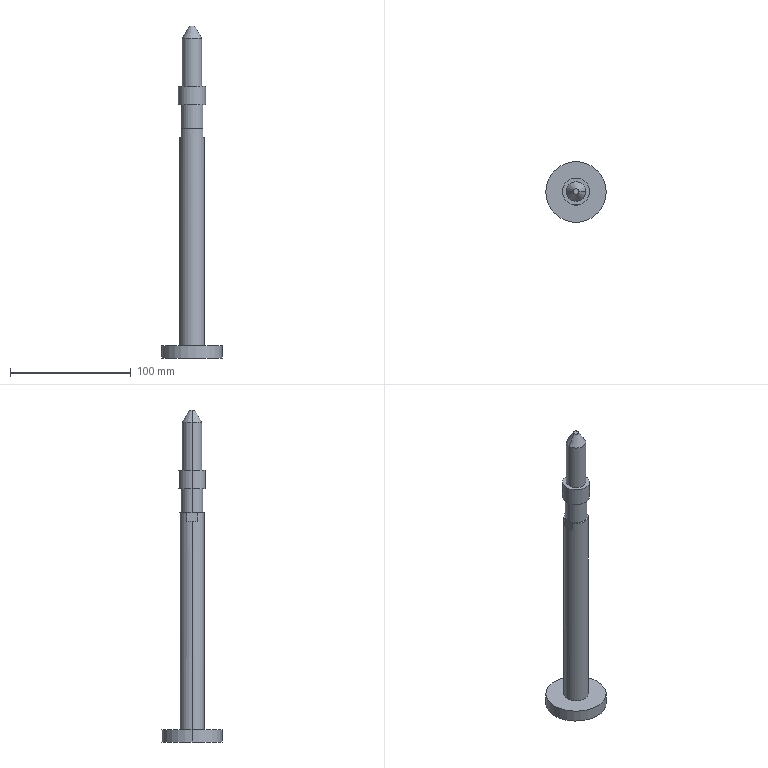Part | STEP file | MB50_125_ROD | 1 solid | 23 faces | box 50 x 50 x 274.5 mm | volume 96086 mm3 | plane 11 | cylinder 10 | cone 2 | commonest cylinder face diameters 16.16 x2 18 x2 20 x2 22.404 x2 50 x2
STEP:
#1=CARTESIAN_POINT('',(0.,0.,0.));
#2=DIRECTION('',(0.,0.,1.));
#3=DIRECTION('',(1.,0.,0.));
#4=AXIS2_PLACEMENT_3D('',#1,#2,#3);
#5=CARTESIAN_POINT('',(2.306,0.,108.));
#6=VERTEX_POINT('',#5);
#7=CARTESIAN_POINT('',(-2.306,0.,108.));
#8=VERTEX_POINT('',#7);
#9=CARTESIAN_POINT('',(0.,0.,108.));
#10=DIRECTION('',(0.,0.,1.));
#11=DIRECTION('',(1.,0.,0.));
#12=AXIS2_PLACEMENT_3D('',#9,#10,#11);
#13=CIRCLE('',#12,2.306);
#14=CARTESIAN_POINT('',(0.,0.,108.));
#15=DIRECTION('',(0.,0.,-1.));
#16=DIRECTION('',(-1.,0.,0.));
#17=AXIS2_PLACEMENT_3D('',#14,#15,#16);
#18=CONICAL_SURFACE('',#17,2.306,0.5236);
#19=CARTESIAN_POINT('',(3.142,0.));
#20=DIRECTION('',(-1.,0.));
#21=VECTOR('',#20,1.);
#22=LINE('',#19,#21);
#23=(GEOMETRIC_REPRESENTATION_CONTEXT(2)PARAMETRIC_REPRESENTATION_CONTEXT()REPRESENTATION_CONTEXT('',''));
#24=DEFINITIONAL_REPRESENTATION('',(#22),#23);
#25=PCURVE('',#18,#24);
#26=CARTESIAN_POINT('',(0.,0.,108.));
#27=DIRECTION('',(0.,0.,1.));
#28=DIRECTION('',(1.,0.,0.));
#29=AXIS2_PLACEMENT_3D('',#26,#27,#28);
#30=PLANE('',#29);
#31=CARTESIAN_POINT('',(0.,0.));
#32=DIRECTION('',(1.,0.));
#33=AXIS2_PLACEMENT_2D('',#31,#32);
#34=CIRCLE('',#33,2.306);
#35=(GEOMETRIC_REPRESENTATION_CONTEXT(2)PARAMETRIC_REPRESENTATION_CONTEXT()REPRESENTATION_CONTEXT('',''));
#36=DEFINITIONAL_REPRESENTATION('',(#34),#35);
#37=PCURVE('',#30,#36);
#38=SURFACE_CURVE('',#13,(#25,#37),.PCURVE_S1.);
#39=EDGE_CURVE('',#6,#8,#38,.T.);
#40=ORIENTED_EDGE('',*,*,#39,.F.);
#41=CARTESIAN_POINT('',(8.08,0.,98.));
#42=VERTEX_POINT('',#41);
#43=CARTESIAN_POINT('',(2.306,0.,108.));
#44=DIRECTION('',(0.5,0.,-0.866));
#45=VECTOR('',#44,1.);
#46=LINE('',#43,#45);
#47=CARTESIAN_POINT('',(3.142,0.));
#48=DIRECTION('',(0.,1.));
#49=VECTOR('',#48,1.);
#50=LINE('',#47,#49);
#51=(GEOMETRIC_REPRESENTATION_CONTEXT(2)PARAMETRIC_REPRESENTATION_CONTEXT()REPRESENTATION_CONTEXT('',''));
#52=DEFINITIONAL_REPRESENTATION('',(#50),#51);
#53=PCURVE('',#18,#52);
#54=CARTESIAN_POINT('',(0.,0.,108.));
#55=DIRECTION('',(0.,0.,-1.));
#56=DIRECTION('',(-1.,0.,0.));
#57=AXIS2_PLACEMENT_3D('',#54,#55,#56);
#58=CONICAL_SURFACE('',#57,2.306,0.5236);
#59=CARTESIAN_POINT('',(3.142,0.));
#60=DIRECTION('',(0.,1.));
#61=VECTOR('',#60,1.);
#62=LINE('',#59,#61);
#63=(GEOMETRIC_REPRESENTATION_CONTEXT(2)PARAMETRIC_REPRESENTATION_CONTEXT()REPRESENTATION_CONTEXT('',''));
#64=DEFINITIONAL_REPRESENTATION('',(#62),#63);
#65=PCURVE('',#58,#64);
#66=SURFACE_CURVE('',#46,(#53,#65),.PCURVE_S1.);
#67=EDGE_CURVE('',#6,#42,#66,.T.);
#68=ORIENTED_EDGE('',*,*,#67,.T.);
#69=CARTESIAN_POINT('',(-8.08,0.,98.));
#70=VERTEX_POINT('',#69);
#71=CARTESIAN_POINT('',(0.,0.,98.));
#72=DIRECTION('',(0.,0.,-1.));
#73=DIRECTION('',(1.,0.,0.));
#74=AXIS2_PLACEMENT_3D('',#71,#72,#73);
#75=CIRCLE('',#74,8.08);
#76=CARTESIAN_POINT('',(-3.142,10.));
#77=DIRECTION('',(1.,0.));
#78=VECTOR('',#77,1.);
#79=LINE('',#76,#78);
#80=(GEOMETRIC_REPRESENTATION_CONTEXT(2)PARAMETRIC_REPRESENTATION_CONTEXT()REPRESENTATION_CONTEXT('',''));
#81=DEFINITIONAL_REPRESENTATION('',(#79),#80);
#82=PCURVE('',#18,#81);
#83=CARTESIAN_POINT('',(0.,0.,108.));
#84=DIRECTION('',(0.,0.,-1.));
#85=DIRECTION('',(-1.,0.,0.));
#86=AXIS2_PLACEMENT_3D('',#83,#84,#85);
#87=CYLINDRICAL_SURFACE('',#86,8.08);
#88=CARTESIAN_POINT('',(-3.142,10.));
#89=DIRECTION('',(1.,0.));
#90=VECTOR('',#89,1.);
#91=LINE('',#88,#90);
#92=(GEOMETRIC_REPRESENTATION_CONTEXT(2)PARAMETRIC_REPRESENTATION_CONTEXT()REPRESENTATION_CONTEXT('',''));
#93=DEFINITIONAL_REPRESENTATION('',(#91),#92);
#94=PCURVE('',#87,#93);
#95=SURFACE_CURVE('',#75,(#82,#94),.PCURVE_S1.);
#96=EDGE_CURVE('',#70,#42,#95,.T.);
#97=ORIENTED_EDGE('',*,*,#96,.F.);
#98=CARTESIAN_POINT('',(-2.306,0.,108.));
#99=DIRECTION('',(-0.5,0.,-0.866));
#100=VECTOR('',#99,1.);
#101=LINE('',#98,#100);
#102=CARTESIAN_POINT('',(0.,0.));
#103=DIRECTION('',(0.,1.));
#104=VECTOR('',#103,1.);
#105=LINE('',#102,#104);
#106=(GEOMETRIC_REPRESENTATION_CONTEXT(2)PARAMETRIC_REPRESENTATION_CONTEXT()REPRESENTATION_CONTEXT('',''));
#107=DEFINITIONAL_REPRESENTATION('',(#105),#106);
#108=PCURVE('',#18,#107);
#109=CARTESIAN_POINT('',(6.283,0.));
#110=DIRECTION('',(0.,1.));
#111=VECTOR('',#110,1.);
#112=LINE('',#109,#111);
#113=(GEOMETRIC_REPRESENTATION_CONTEXT(2)PARAMETRIC_REPRESENTATION_CONTEXT()REPRESENTATION_CONTEXT('',''));
#114=DEFINITIONAL_REPRESENTATION('',(#112),#113);
#115=PCURVE('',#58,#114);
#116=SURFACE_CURVE('',#101,(#108,#115),.PCURVE_S1.);
#117=EDGE_CURVE('',#8,#70,#116,.T.);
#118=ORIENTED_EDGE('',*,*,#117,.F.);
#119=EDGE_LOOP('',(#40,#68,#97,#118));
#120=FACE_BOUND('',#119,.T.);
#121=ADVANCED_FACE('',(#120),#18,.T.);
#122=ORIENTED_EDGE('',*,*,#96,.T.);
#123=CARTESIAN_POINT('',(8.08,0.,58.));
#124=VERTEX_POINT('',#123);
#125=CARTESIAN_POINT('',(8.08,0.,108.));
#126=DIRECTION('',(0.,0.,-1.));
#127=VECTOR('',#126,1.);
#128=LINE('',#125,#127);
#129=CARTESIAN_POINT('',(3.142,0.));
#130=DIRECTION('',(0.,1.));
#131=VECTOR('',#130,1.);
#132=LINE('',#129,#131);
#133=(GEOMETRIC_REPRESENTATION_CONTEXT(2)PARAMETRIC_REPRESENTATION_CONTEXT()REPRESENTATION_CONTEXT('',''));
#134=DEFINITIONAL_REPRESENTATION('',(#132),#133);
#135=PCURVE('',#87,#134);
#136=CARTESIAN_POINT('',(0.,0.,108.));
#137=DIRECTION('',(0.,0.,-1.));
#138=DIRECTION('',(-1.,0.,0.));
#139=AXIS2_PLACEMENT_3D('',#136,#137,#138);
#140=CYLINDRICAL_SURFACE('',#139,8.08);
#141=CARTESIAN_POINT('',(3.142,0.));
#142=DIRECTION('',(0.,1.));
#143=VECTOR('',#142,1.);
#144=LINE('',#141,#143);
#145=(GEOMETRIC_REPRESENTATION_CONTEXT(2)PARAMETRIC_REPRESENTATION_CONTEXT()REPRESENTATION_CONTEXT('',''));
#146=DEFINITIONAL_REPRESENTATION('',(#144),#145);
#147=PCURVE('',#140,#146);
#148=SURFACE_CURVE('',#128,(#135,#147),.PCURVE_S1.);
#149=EDGE_CURVE('',#42,#124,#148,.T.);
#150=ORIENTED_EDGE('',*,*,#149,.T.);
#151=CARTESIAN_POINT('',(-8.08,0.,58.));
#152=VERTEX_POINT('',#151);
#153=CARTESIAN_POINT('',(0.,0.,58.));
#154=DIRECTION('',(0.,0.,1.));
#155=DIRECTION('',(1.,0.,0.));
#156=AXIS2_PLACEMENT_3D('',#153,#154,#155);
#157=CIRCLE('',#156,8.08);
#158=CARTESIAN_POINT('',(3.142,50.));
#159=DIRECTION('',(-1.,0.));
#160=VECTOR('',#159,1.);
#161=LINE('',#158,#160);
#162=(GEOMETRIC_REPRESENTATION_CONTEXT(2)PARAMETRIC_REPRESENTATION_CONTEXT()REPRESENTATION_CONTEXT('',''));
#163=DEFINITIONAL_REPRESENTATION('',(#161),#162);
#164=PCURVE('',#87,#163);
#165=CARTESIAN_POINT('',(0.,0.,58.));
#166=DIRECTION('',(0.,0.,1.));
#167=DIRECTION('',(1.,0.,0.));
#168=AXIS2_PLACEMENT_3D('',#165,#166,#167);
#169=PLANE('',#168);
#170=CARTESIAN_POINT('',(0.,0.));
#171=DIRECTION('',(1.,0.));
#172=AXIS2_PLACEMENT_2D('',#170,#171);
#173=CIRCLE('',#172,8.08);
#174=(GEOMETRIC_REPRESENTATION_CONTEXT(2)PARAMETRIC_REPRESENTATION_CONTEXT()REPRESENTATION_CONTEXT('',''));
#175=DEFINITIONAL_REPRESENTATION('',(#173),#174);
#176=PCURVE('',#169,#175);
#177=SURFACE_CURVE('',#157,(#164,#176),.PCURVE_S1.);
#178=EDGE_CURVE('',#124,#152,#177,.T.);
#179=ORIENTED_EDGE('',*,*,#178,.T.);
#180=CARTESIAN_POINT('',(-8.08,0.,108.));
#181=DIRECTION('',(0.,0.,-1.));
#182=VECTOR('',#181,1.);
#183=LINE('',#180,#182);
#184=CARTESIAN_POINT('',(0.,0.));
#185=DIRECTION('',(0.,1.));
#186=VECTOR('',#185,1.);
#187=LINE('',#184,#186);
#188=(GEOMETRIC_REPRESENTATION_CONTEXT(2)PARAMETRIC_REPRESENTATION_CONTEXT()REPRESENTATION_CONTEXT('',''));
#189=DEFINITIONAL_REPRESENTATION('',(#187),#188);
#190=PCURVE('',#87,#189);
#191=CARTESIAN_POINT('',(6.283,0.));
#192=DIRECTION('',(0.,1.));
#193=VECTOR('',#192,1.);
#194=LINE('',#191,#193);
#195=(GEOMETRIC_REPRESENTATION_CONTEXT(2)PARAMETRIC_REPRESENTATION_CONTEXT()REPRESENTATION_CONTEXT('',''));
#196=DEFINITIONAL_REPRESENTATION('',(#194),#195);
#197=PCURVE('',#140,#196);
#198=SURFACE_CURVE('',#183,(#190,#197),.PCURVE_S1.);
#199=EDGE_CURVE('',#70,#152,#198,.T.);
#200=ORIENTED_EDGE('',*,*,#199,.F.);
#201=EDGE_LOOP('',(#122,#150,#179,#200));
#202=FACE_BOUND('',#201,.T.);
#203=ADVANCED_FACE('',(#202),#87,.T.);
#204=CARTESIAN_POINT('',(11.202,0.,43.));
#205=VERTEX_POINT('',#204);
#206=CARTESIAN_POINT('',(-11.202,0.,43.));
#207=VERTEX_POINT('',#206);
#208=CARTESIAN_POINT('',(0.,0.,43.));
#209=DIRECTION('',(0.,0.,1.));
#210=DIRECTION('',(1.,0.,0.));
#211=AXIS2_PLACEMENT_3D('',#208,#209,#210);
#212=CIRCLE('',#211,11.202);
#213=CARTESIAN_POINT('',(0.,0.,43.));
#214=DIRECTION('',(0.,0.,1.));
#215=DIRECTION('',(1.,0.,0.));
#216=AXIS2_PLACEMENT_3D('',#213,#214,#215);
#217=CYLINDRICAL_SURFACE('',#216,11.202);
#218=CARTESIAN_POINT('',(0.,0.));
#219=DIRECTION('',(1.,0.));
#220=VECTOR('',#219,1.);
#221=LINE('',#218,#220);
#222=(GEOMETRIC_REPRESENTATION_CONTEXT(2)PARAMETRIC_REPRESENTATION_CONTEXT()REPRESENTATION_CONTEXT('',''));
#223=DEFINITIONAL_REPRESENTATION('',(#221),#222);
#224=PCURVE('',#217,#223);
#225=CARTESIAN_POINT('',(0.,0.,43.));
#226=DIRECTION('',(0.,0.,1.));
#227=DIRECTION('',(1.,0.,0.));
#228=AXIS2_PLACEMENT_3D('',#225,#226,#227);
#229=PLANE('',#228);
#230=CARTESIAN_POINT('',(0.,0.));
#231=DIRECTION('',(1.,0.));
#232=AXIS2_PLACEMENT_2D('',#230,#231);
#233=CIRCLE('',#232,11.202);
#234=(GEOMETRIC_REPRESENTATION_CONTEXT(2)PARAMETRIC_REPRESENTATION_CONTEXT()REPRESENTATION_CONTEXT('',''));
#235=DEFINITIONAL_REPRESENTATION('',(#233),#234);
#236=PCURVE('',#229,#235);
#237=SURFACE_CURVE('',#212,(#224,#236),.PCURVE_S1.);
#238=EDGE_CURVE('',#205,#207,#237,.T.);
#239=ORIENTED_EDGE('',*,*,#238,.T.);
#240=CARTESIAN_POINT('',(-11.202,0.,58.));
#241=VERTEX_POINT('',#240);
#242=CARTESIAN_POINT('',(-11.202,0.,43.));
#243=DIRECTION('',(0.,0.,1.));
#244=VECTOR('',#243,1.);
#245=LINE('',#242,#244);
#246=CARTESIAN_POINT('',(3.142,0.));
#247=DIRECTION('',(0.,1.));
#248=VECTOR('',#247,1.);
#249=LINE('',#246,#248);
#250=(GEOMETRIC_REPRESENTATION_CONTEXT(2)PARAMETRIC_REPRESENTATION_CONTEXT()REPRESENTATION_CONTEXT('',''));
#251=DEFINITIONAL_REPRESENTATION('',(#249),#250);
#252=PCURVE('',#217,#251);
#253=CARTESIAN_POINT('',(0.,0.,43.));
#254=DIRECTION('',(0.,0.,1.));
#255=DIRECTION('',(1.,0.,0.));
#256=AXIS2_PLACEMENT_3D('',#253,#254,#255);
#257=CYLINDRICAL_SURFACE('',#256,11.202);
#258=CARTESIAN_POINT('',(3.142,0.));
#259=DIRECTION('',(0.,1.));
#260=VECTOR('',#259,1.);
#261=LINE('',#258,#260);
#262=(GEOMETRIC_REPRESENTATION_CONTEXT(2)PARAMETRIC_REPRESENTATION_CONTEXT()REPRESENTATION_CONTEXT('',''));
#263=DEFINITIONAL_REPRESENTATION('',(#261),#262);
#264=PCURVE('',#257,#263);
#265=SURFACE_CURVE('',#245,(#252,#264),.PCURVE_S1.);
#266=EDGE_CURVE('',#207,#241,#265,.T.);
#267=ORIENTED_EDGE('',*,*,#266,.T.);
#268=CARTESIAN_POINT('',(11.202,0.,58.));
#269=VERTEX_POINT('',#268);
#270=CARTESIAN_POINT('',(0.,0.,58.));
#271=DIRECTION('',(0.,0.,1.));
#272=DIRECTION('',(1.,0.,0.));
#273=AXIS2_PLACEMENT_3D('',#270,#271,#272);
#274=CIRCLE('',#273,11.202);
#275=CARTESIAN_POINT('',(0.,15.));
#276=DIRECTION('',(1.,0.));
#277=VECTOR('',#276,1.);
#278=LINE('',#275,#277);
#279=(GEOMETRIC_REPRESENTATION_CONTEXT(2)PARAMETRIC_REPRESENTATION_CONTEXT()REPRESENTATION_CONTEXT('',''));
#280=DEFINITIONAL_REPRESENTATION('',(#278),#279);
#281=PCURVE('',#217,#280);
#282=CARTESIAN_POINT('',(0.,0.));
#283=DIRECTION('',(1.,0.));
#284=AXIS2_PLACEMENT_2D('',#282,#283);
#285=CIRCLE('',#284,11.202);
#286=(GEOMETRIC_REPRESENTATION_CONTEXT(2)PARAMETRIC_REPRESENTATION_CONTEXT()REPRESENTATION_CONTEXT('',''));
#287=DEFINITIONAL_REPRESENTATION('',(#285),#286);
#288=PCURVE('',#169,#287);
#289=SURFACE_CURVE('',#274,(#281,#288),.PCURVE_S1.);
#290=EDGE_CURVE('',#269,#241,#289,.T.);
#291=ORIENTED_EDGE('',*,*,#290,.F.);
#292=CARTESIAN_POINT('',(11.202,0.,43.));
#293=DIRECTION('',(0.,0.,1.));
#294=VECTOR('',#293,1.);
#295=LINE('',#292,#294);
#296=CARTESIAN_POINT('',(0.,0.));
#297=DIRECTION('',(0.,1.));
#298=VECTOR('',#297,1.);
#299=LINE('',#296,#298);
#300=(GEOMETRIC_REPRESENTATION_CONTEXT(2)PARAMETRIC_REPRESENTATION_CONTEXT()REPRESENTATION_CONTEXT('',''));
#301=DEFINITIONAL_REPRESENTATION('',(#299),#300);
#302=PCURVE('',#217,#301);
#303=CARTESIAN_POINT('',(6.283,0.));
#304=DIRECTION('',(0.,1.));
#305=VECTOR('',#304,1.);
#306=LINE('',#303,#305);
#307=(GEOMETRIC_REPRESENTATION_CONTEXT(2)PARAMETRIC_REPRESENTATION_CONTEXT()REPRESENTATION_CONTEXT('',''));
#308=DEFINITIONAL_REPRESENTATION('',(#306),#307);
#309=PCURVE('',#257,#308);
#310=SURFACE_CURVE('',#295,(#302,#309),.PCURVE_S1.);
#311=EDGE_CURVE('',#205,#269,#310,.T.);
#312=ORIENTED_EDGE('',*,*,#311,.F.);
#313=EDGE_LOOP('',(#239,#267,#291,#312));
#314=FACE_BOUND('',#313,.T.);
#315=ADVANCED_FACE('',(#314),#217,.T.);
#316=CARTESIAN_POINT('',(25.,0.,-166.5));
#317=VERTEX_POINT('',#316);
#318=CARTESIAN_POINT('',(-25.,0.,-166.5));
#319=VERTEX_POINT('',#318);
#320=CARTESIAN_POINT('',(0.,0.,-166.5));
#321=DIRECTION('',(0.,0.,1.));
#322=DIRECTION('',(1.,0.,0.));
#323=AXIS2_PLACEMENT_3D('',#320,#321,#322);
#324=CIRCLE('',#323,25.);
#325=CARTESIAN_POINT('',(0.,0.,-166.5));
#326=DIRECTION('',(0.,0.,1.));
#327=DIRECTION('',(1.,0.,0.));
#328=AXIS2_PLACEMENT_3D('',#325,#326,#327);
#329=CYLINDRICAL_SURFACE('',#328,25.);
#330=CARTESIAN_POINT('',(0.,0.));
#331=DIRECTION('',(1.,0.));
#332=VECTOR('',#331,1.);
#333=LINE('',#330,#332);
#334=(GEOMETRIC_REPRESENTATION_CONTEXT(2)PARAMETRIC_REPRESENTATION_CONTEXT()REPRESENTATION_CONTEXT('',''));
#335=DEFINITIONAL_REPRESENTATION('',(#333),#334);
#336=PCURVE('',#329,#335);
#337=CARTESIAN_POINT('',(0.,25.,-166.5));
#338=DIRECTION('',(0.,0.,1.));
#339=DIRECTION('',(1.,0.,0.));
#340=AXIS2_PLACEMENT_3D('',#337,#338,#339);
#341=PLANE('',#340);
#342=CARTESIAN_POINT('',(0.,-25.));
#343=DIRECTION('',(1.,0.));
#344=AXIS2_PLACEMENT_2D('',#342,#343);
#345=CIRCLE('',#344,25.);
#346=(GEOMETRIC_REPRESENTATION_CONTEXT(2)PARAMETRIC_REPRESENTATION_CONTEXT()REPRESENTATION_CONTEXT('',''));
#347=DEFINITIONAL_REPRESENTATION('',(#345),#346);
#348=PCURVE('',#341,#347);
#349=SURFACE_CURVE('',#324,(#336,#348),.PCURVE_S1.);
#350=EDGE_CURVE('',#317,#319,#349,.T.);
#351=ORIENTED_EDGE('',*,*,#350,.T.);
#352=CARTESIAN_POINT('',(-25.,0.,-156.5));
#353=VERTEX_POINT('',#352);
#354=CARTESIAN_POINT('',(-25.,0.,-166.5));
#355=DIRECTION('',(0.,0.,1.));
#356=VECTOR('',#355,1.);
#357=LINE('',#354,#356);
#358=CARTESIAN_POINT('',(3.142,0.));
#359=DIRECTION('',(0.,1.));
#360=VECTOR('',#359,1.);
#361=LINE('',#358,#360);
#362=(GEOMETRIC_REPRESENTATION_CONTEXT(2)PARAMETRIC_REPRESENTATION_CONTEXT()REPRESENTATION_CONTEXT('',''));
#363=DEFINITIONAL_REPRESENTATION('',(#361),#362);
#364=PCURVE('',#329,#363);
#365=CARTESIAN_POINT('',(0.,0.,-166.5));
#366=DIRECTION('',(0.,0.,1.));
#367=DIRECTION('',(1.,0.,0.));
#368=AXIS2_PLACEMENT_3D('',#365,#366,#367);
#369=CYLINDRICAL_SURFACE('',#368,25.);
#370=CARTESIAN_POINT('',(3.142,0.));
#371=DIRECTION('',(0.,1.));
#372=VECTOR('',#371,1.);
#373=LINE('',#370,#372);
#374=(GEOMETRIC_REPRESENTATION_CONTEXT(2)PARAMETRIC_REPRESENTATION_CONTEXT()REPRESENTATION_CONTEXT('',''));
#375=DEFINITIONAL_REPRESENTATION('',(#373),#374);
#376=PCURVE('',#369,#375);
#377=SURFACE_CURVE('',#357,(#364,#376),.PCURVE_S1.);
#378=EDGE_CURVE('',#319,#353,#377,.T.);
#379=ORIENTED_EDGE('',*,*,#378,.T.);
#380=CARTESIAN_POINT('',(25.,0.,-156.5));
#381=VERTEX_POINT('',#380);
#382=CARTESIAN_POINT('',(0.,0.,-156.5));
#383=DIRECTION('',(0.,0.,1.));
#384=DIRECTION('',(1.,0.,0.));
#385=AXIS2_PLACEMENT_3D('',#382,#383,#384);
#386=CIRCLE('',#385,25.);
#387=CARTESIAN_POINT('',(0.,10.));
#388=DIRECTION('',(1.,0.));
#389=VECTOR('',#388,1.);
#390=LINE('',#387,#389);
#391=(GEOMETRIC_REPRESENTATION_CONTEXT(2)PARAMETRIC_REPRESENTATION_CONTEXT()REPRESENTATION_CONTEXT('',''));
#392=DEFINITIONAL_REPRESENTATION('',(#390),#391);
#393=PCURVE('',#329,#392);
#394=CARTESIAN_POINT('',(0.,10.,-156.5));
#395=DIRECTION('',(0.,0.,-1.));
#396=DIRECTION('',(-1.,0.,0.));
#397=AXIS2_PLACEMENT_3D('',#394,#395,#396);
#398=PLANE('',#397);
#399=CARTESIAN_POINT('',(-25.,-10.));
#400=CARTESIAN_POINT('',(-25.,33.301));
#401=CARTESIAN_POINT('',(12.5,11.651));
#402=CARTESIAN_POINT('',(50.,-10.));
#403=CARTESIAN_POINT('',(12.5,-31.651));
#404=CARTESIAN_POINT('',(-25.,-53.301));
#405=CARTESIAN_POINT('',(-25.,-10.));
#406=(BOUNDED_CURVE()B_SPLINE_CURVE(2,(#399,#400,#401,#402,#403,#404,#405),.UNSPECIFIED.,.T.,.F.)B_SPLINE_CURVE_WITH_KNOTS((1,2,2,2,2,1),(-2.094,0.,2.094,4.189,6.283,8.378),.UNSPECIFIED.)CURVE()GEOMETRIC_REPRESENTATION_ITEM()RATIONAL_B_SPLINE_CURVE((1.,0.5,1.,0.5,1.,0.5,1.))REPRESENTATION_ITEM(''));
#407=(GEOMETRIC_REPRESENTATION_CONTEXT(2)PARAMETRIC_REPRESENTATION_CONTEXT()REPRESENTATION_CONTEXT('',''));
#408=DEFINITIONAL_REPRESENTATION('',(#406),#407);
#409=PCURVE('',#398,#408);
#410=SURFACE_CURVE('',#386,(#393,#409),.PCURVE_S1.);
#411=EDGE_CURVE('',#381,#353,#410,.T.);
#412=ORIENTED_EDGE('',*,*,#411,.F.);
#413=CARTESIAN_POINT('',(25.,0.,-166.5));
#414=DIRECTION('',(0.,0.,1.));
#415=VECTOR('',#414,1.);
#416=LINE('',#413,#415);
#417=CARTESIAN_POINT('',(0.,0.));
#418=DIRECTION('',(0.,1.));
#419=VECTOR('',#418,1.);
#420=LINE('',#417,#419);
#421=(GEOMETRIC_REPRESENTATION_CONTEXT(2)PARAMETRIC_REPRESENTATION_CONTEXT()REPRESENTATION_CONTEXT('',''));
#422=DEFINITIONAL_REPRESENTATION('',(#420),#421);
#423=PCURVE('',#329,#422);
#424=CARTESIAN_POINT('',(6.283,0.));
#425=DIRECTION('',(0.,1.));
#426=VECTOR('',#425,1.);
#427=LINE('',#424,#426);
#428=(GEOMETRIC_REPRESENTATION_CONTEXT(2)PARAMETRIC_REPRESENTATION_CONTEXT()REPRESENTATION_CONTEXT('',''));
#429=DEFINITIONAL_REPRESENTATION('',(#427),#428);
#430=PCURVE('',#369,#429);
#431=SURFACE_CURVE('',#416,(#423,#430),.PCURVE_S1.);
#432=EDGE_CURVE('',#317,#381,#431,.T.);
#433=ORIENTED_EDGE('',*,*,#432,.F.);
#434=EDGE_LOOP('',(#351,#379,#412,#433));
#435=FACE_BOUND('',#434,.T.);
#436=ADVANCED_FACE('',(#435),#329,.T.);
#437=CARTESIAN_POINT('',(10.,0.,-156.5));
#438=VERTEX_POINT('',#437);
#439=CARTESIAN_POINT('',(-10.,0.,-156.5));
#440=VERTEX_POINT('',#439);
#441=CARTESIAN_POINT('',(0.,0.,-156.5));
#442=DIRECTION('',(0.,0.,1.));
#443=DIRECTION('',(1.,0.,0.));
#444=AXIS2_PLACEMENT_3D('',#441,#442,#443);
#445=CIRCLE('',#444,10.);
#446=CARTESIAN_POINT('',(0.,0.,-166.5));
#447=DIRECTION('',(0.,0.,1.));
#448=DIRECTION('',(1.,0.,0.));
#449=AXIS2_PLACEMENT_3D('',#446,#447,#448);
#450=CYLINDRICAL_SURFACE('',#449,10.);
#451=CARTESIAN_POINT('',(0.,10.));
#452=DIRECTION('',(1.,0.));
#453=VECTOR('',#452,1.);
#454=LINE('',#451,#453);
#455=(GEOMETRIC_REPRESENTATION_CONTEXT(2)PARAMETRIC_REPRESENTATION_CONTEXT()REPRESENTATION_CONTEXT('',''));
#456=DEFINITIONAL_REPRESENTATION('',(#454),#455);
#457=PCURVE('',#450,#456);
#458=CARTESIAN_POINT('',(-10.,-10.));
#459=CARTESIAN_POINT('',(-10.,7.321));
#460=CARTESIAN_POINT('',(5.,-1.34));
#461=CARTESIAN_POINT('',(20.,-10.));
#462=CARTESIAN_POINT('',(5.,-18.66));
#463=CARTESIAN_POINT('',(-10.,-27.321));
#464=CARTESIAN_POINT('',(-10.,-10.));
#465=(BOUNDED_CURVE()B_SPLINE_CURVE(2,(#458,#459,#460,#461,#462,#463,#464),.UNSPECIFIED.,.T.,.F.)B_SPLINE_CURVE_WITH_KNOTS((1,2,2,2,2,1),(-2.094,0.,2.094,4.189,6.283,8.378),.UNSPECIFIED.)CURVE()GEOMETRIC_REPRESENTATION_ITEM()RATIONAL_B_SPLINE_CURVE((1.,0.5,1.,0.5,1.,0.5,1.))REPRESENTATION_ITEM(''));
#466=(GEOMETRIC_REPRESENTATION_CONTEXT(2)PARAMETRIC_REPRESENTATION_CONTEXT()REPRESENTATION_CONTEXT('',''));
#467=DEFINITIONAL_REPRESENTATION('',(#465),#466);
#468=PCURVE('',#398,#467);
#469=SURFACE_CURVE('',#445,(#457,#468),.PCURVE_S1.);
#470=EDGE_CURVE('',#438,#440,#469,.T.);
#471=ORIENTED_EDGE('',*,*,#470,.T.);
#472=CARTESIAN_POINT('',(-10.,0.,16.));
#473=VERTEX_POINT('',#472);
#474=CARTESIAN_POINT('',(-10.,0.,-166.5));
#475=DIRECTION('',(0.,0.,1.));
#476=VECTOR('',#475,1.);
#477=LINE('',#474,#476);
#478=CARTESIAN_POINT('',(3.142,0.));
#479=DIRECTION('',(0.,1.));
#480=VECTOR('',#479,1.);
#481=LINE('',#478,#480);
#482=(GEOMETRIC_REPRESENTATION_CONTEXT(2)PARAMETRIC_REPRESENTATION_CONTEXT()REPRESENTATION_CONTEXT('',''));
#483=DEFINITIONAL_REPRESENTATION('',(#481),#482);
#484=PCURVE('',#450,#483);
#485=CARTESIAN_POINT('',(0.,0.,-166.5));
#486=DIRECTION('',(0.,0.,1.));
#487=DIRECTION('',(1.,0.,0.));
#488=AXIS2_PLACEMENT_3D('',#485,#486,#487);
#489=CYLINDRICAL_SURFACE('',#488,10.);
#490=CARTESIAN_POINT('',(3.142,0.));
#491=DIRECTION('',(0.,1.));
#492=VECTOR('',#491,1.);
#493=LINE('',#490,#492);
#494=(GEOMETRIC_REPRESENTATION_CONTEXT(2)PARAMETRIC_REPRESENTATION_CONTEXT()REPRESENTATION_CONTEXT('',''));
#495=DEFINITIONAL_REPRESENTATION('',(#493),#494);
#496=PCURVE('',#489,#495);
#497=SURFACE_CURVE('',#477,(#484,#496),.PCURVE_S1.);
#498=EDGE_CURVE('',#440,#473,#497,.T.);
#499=ORIENTED_EDGE('',*,*,#498,.T.);
#500=CARTESIAN_POINT('',(-9.,4.359,16.));
#501=VERTEX_POINT('',#500);
#502=CARTESIAN_POINT('',(0.,0.,16.));
#503=DIRECTION('',(0.,0.,1.));
#504=DIRECTION('',(1.,0.,0.));
#505=AXIS2_PLACEMENT_3D('',#502,#503,#504);
#506=CIRCLE('',#505,10.);
#507=CARTESIAN_POINT('',(0.,182.5));
#508=DIRECTION('',(1.,0.));
#509=VECTOR('',#508,1.);
#510=LINE('',#507,#509);
#511=(GEOMETRIC_REPRESENTATION_CONTEXT(2)PARAMETRIC_REPRESENTATION_CONTEXT()REPRESENTATION_CONTEXT('',''));
#512=DEFINITIONAL_REPRESENTATION('',(#510),#511);
#513=PCURVE('',#450,#512);
#514=CARTESIAN_POINT('',(0.,0.,16.));
#515=DIRECTION('',(0.,0.,1.));
#516=DIRECTION('',(1.,0.,0.));
#517=AXIS2_PLACEMENT_3D('',#514,#515,#516);
#518=PLANE('',#517);
#519=CARTESIAN_POINT('',(0.,0.));
#520=DIRECTION('',(1.,0.));
#521=AXIS2_PLACEMENT_2D('',#519,#520);
#522=CIRCLE('',#521,10.);
#523=(GEOMETRIC_REPRESENTATION_CONTEXT(2)PARAMETRIC_REPRESENTATION_CONTEXT()REPRESENTATION_CONTEXT('',''));
#524=DEFINITIONAL_REPRESENTATION('',(#522),#523);
#525=PCURVE('',#518,#524);
#526=SURFACE_CURVE('',#506,(#513,#525),.PCURVE_S1.);
#527=EDGE_CURVE('',#501,#473,#526,.T.);
#528=ORIENTED_EDGE('',*,*,#527,.F.);
#529=CARTESIAN_POINT('',(-9.,4.359,23.));
#530=VERTEX_POINT('',#529);
#531=CARTESIAN_POINT('',(-9.,4.359,16.));
#532=DIRECTION('',(0.,0.,1.));
#533=VECTOR('',#532,1.);
#534=LINE('',#531,#533);
#535=CARTESIAN_POINT('',(2.691,182.5));
#536=DIRECTION('',(0.,1.));
#537=VECTOR('',#536,1.);
#538=LINE('',#535,#537);
#539=(GEOMETRIC_REPRESENTATION_CONTEXT(2)PARAMETRIC_REPRESENTATION_CONTEXT()REPRESENTATION_CONTEXT('',''));
#540=DEFINITIONAL_REPRESENTATION('',(#538),#539);
#541=PCURVE('',#450,#540);
#542=CARTESIAN_POINT('',(-9.,4.359,16.));
#543=DIRECTION('',(-1.,0.,0.));
#544=DIRECTION('',(0.,0.,1.));
#545=AXIS2_PLACEMENT_3D('',#542,#543,#544);
#546=PLANE('',#545);
#547=CARTESIAN_POINT('',(0.,0.));
#548=DIRECTION('',(1.,0.));
#549=VECTOR('',#548,1.);
#550=LINE('',#547,#549);
#551=(GEOMETRIC_REPRESENTATION_CONTEXT(2)PARAMETRIC_REPRESENTATION_CONTEXT()REPRESENTATION_CONTEXT('',''));
#552=DEFINITIONAL_REPRESENTATION('',(#550),#551);
#553=PCURVE('',#546,#552);
#554=SURFACE_CURVE('',#534,(#541,#553),.PCURVE_S1.);
#555=EDGE_CURVE('',#501,#530,#554,.T.);
#556=ORIENTED_EDGE('',*,*,#555,.T.);
#557=CARTESIAN_POINT('',(9.,4.359,23.));
#558=VERTEX_POINT('',#557);
#559=CARTESIAN_POINT('',(0.,0.,23.));
#560=DIRECTION('',(0.,0.,1.));
#561=DIRECTION('',(1.,0.,0.));
#562=AXIS2_PLACEMENT_3D('',#559,#560,#561);
#563=CIRCLE('',#562,10.);
#564=CARTESIAN_POINT('',(0.,189.5));
#565=DIRECTION('',(1.,0.));
#566=VECTOR('',#565,1.);
#567=LINE('',#564,#566);
#568=(GEOMETRIC_REPRESENTATION_CONTEXT(2)PARAMETRIC_REPRESENTATION_CONTEXT()REPRESENTATION_CONTEXT('',''));
#569=DEFINITIONAL_REPRESENTATION('',(#567),#568);
#570=PCURVE('',#450,#569);
#571=CARTESIAN_POINT('',(0.,9.,23.));
#572=DIRECTION('',(0.,0.,-1.));
#573=DIRECTION('',(-1.,0.,0.));
#574=AXIS2_PLACEMENT_3D('',#571,#572,#573);
#575=PLANE('',#574);
#576=CARTESIAN_POINT('',(-10.,-9.));
#577=CARTESIAN_POINT('',(-10.,8.321));
#578=CARTESIAN_POINT('',(5.,-0.3397));
#579=CARTESIAN_POINT('',(20.,-9.));
#580=CARTESIAN_POINT('',(5.,-17.66));
#581=CARTESIAN_POINT('',(-10.,-26.321));
#582=CARTESIAN_POINT('',(-10.,-9.));
#583=(BOUNDED_CURVE()B_SPLINE_CURVE(2,(#576,#577,#578,#579,#580,#581,#582),.UNSPECIFIED.,.T.,.F.)B_SPLINE_CURVE_WITH_KNOTS((1,2,2,2,2,1),(-2.094,0.,2.094,4.189,6.283,8.378),.UNSPECIFIED.)CURVE()GEOMETRIC_REPRESENTATION_ITEM()RATIONAL_B_SPLINE_CURVE((1.,0.5,1.,0.5,1.,0.5,1.))REPRESENTATION_ITEM(''));
#584=(GEOMETRIC_REPRESENTATION_CONTEXT(2)PARAMETRIC_REPRESENTATION_CONTEXT()REPRESENTATION_CONTEXT('',''));
#585=DEFINITIONAL_REPRESENTATION('',(#583),#584);
#586=PCURVE('',#575,#585);
#587=SURFACE_CURVE('',#563,(#570,#586),.PCURVE_S1.);
#588=EDGE_CURVE('',#558,#530,#587,.T.);
#589=ORIENTED_EDGE('',*,*,#588,.F.);
#590=CARTESIAN_POINT('',(9.,4.359,16.));
#591=VERTEX_POINT('',#590);
#592=CARTESIAN_POINT('',(9.,4.359,16.));
#593=DIRECTION('',(0.,0.,1.));
#594=VECTOR('',#593,1.);
#595=LINE('',#592,#594);
#596=CARTESIAN_POINT('',(0.451,182.5));
#597=DIRECTION('',(0.,1.));
#598=VECTOR('',#597,1.);
#599=LINE('',#596,#598);
#600=(GEOMETRIC_REPRESENTATION_CONTEXT(2)PARAMETRIC_REPRESENTATION_CONTEXT()REPRESENTATION_CONTEXT('',''));
#601=DEFINITIONAL_REPRESENTATION('',(#599),#600);
#602=PCURVE('',#450,#601);
#603=CARTESIAN_POINT('',(9.,-4.359,16.));
#604=DIRECTION('',(1.,0.,0.));
#605=DIRECTION('',(0.,0.,-1.));
#606=AXIS2_PLACEMENT_3D('',#603,#604,#605);
#607=PLANE('',#606);
#608=CARTESIAN_POINT('',(0.,8.718));
#609=DIRECTION('',(-1.,0.));
#610=VECTOR('',#609,1.);
#611=LINE('',#608,#610);
#612=(GEOMETRIC_REPRESENTATION_CONTEXT(2)PARAMETRIC_REPRESENTATION_CONTEXT()REPRESENTATION_CONTEXT('',''));
#613=DEFINITIONAL_REPRESENTATION('',(#611),#612);
#614=PCURVE('',#607,#613);
#615=SURFACE_CURVE('',#595,(#602,#614),.PCURVE_S1.);
#616=EDGE_CURVE('',#591,#558,#615,.T.);
#617=ORIENTED_EDGE('',*,*,#616,.F.);
#618=CARTESIAN_POINT('',(10.,0.,16.));
#619=VERTEX_POINT('',#618);
#620=CARTESIAN_POINT('',(0.,0.,16.));
#621=DIRECTION('',(0.,0.,1.));
#622=DIRECTION('',(1.,0.,0.));
#623=AXIS2_PLACEMENT_3D('',#620,#621,#622);
#624=CIRCLE('',#623,10.);
#625=CARTESIAN_POINT('',(0.,182.5));
#626=DIRECTION('',(1.,0.));
#627=VECTOR('',#626,1.);
#628=LINE('',#625,#627);
#629=(GEOMETRIC_REPRESENTATION_CONTEXT(2)PARAMETRIC_REPRESENTATION_CONTEXT()REPRESENTATION_CONTEXT('',''));
#630=DEFINITIONAL_REPRESENTATION('',(#628),#629);
#631=PCURVE('',#450,#630);
#632=CARTESIAN_POINT('',(0.,0.,16.));
#633=DIRECTION('',(0.,0.,1.));
#634=DIRECTION('',(1.,0.,0.));
#635=AXIS2_PLACEMENT_3D('',#632,#633,#634);
#636=PLANE('',#635);
#637=CARTESIAN_POINT('',(0.,0.));
#638=DIRECTION('',(1.,0.));
#639=AXIS2_PLACEMENT_2D('',#637,#638);
#640=CIRCLE('',#639,10.);
#641=(GEOMETRIC_REPRESENTATION_CONTEXT(2)PARAMETRIC_REPRESENTATION_CONTEXT()REPRESENTATION_CONTEXT('',''));
#642=DEFINITIONAL_REPRESENTATION('',(#640),#641);
#643=PCURVE('',#636,#642);
#644=SURFACE_CURVE('',#624,(#631,#643),.PCURVE_S1.);
#645=EDGE_CURVE('',#619,#591,#644,.T.);
#646=ORIENTED_EDGE('',*,*,#645,.F.);
#647=CARTESIAN_POINT('',(10.,0.,-166.5));
#648=DIRECTION('',(0.,0.,1.));
#649=VECTOR('',#648,1.);
#650=LINE('',#647,#649);
#651=CARTESIAN_POINT('',(0.,0.));
#652=DIRECTION('',(0.,1.));
#653=VECTOR('',#652,1.);
#654=LINE('',#651,#653);
#655=(GEOMETRIC_REPRESENTATION_CONTEXT(2)PARAMETRIC_REPRESENTATION_CONTEXT()REPRESENTATION_CONTEXT('',''));
#656=DEFINITIONAL_REPRESENTATION('',(#654),#655);
#657=PCURVE('',#450,#656);
#658=CARTESIAN_POINT('',(6.283,0.));
#659=DIRECTION('',(0.,1.));
#660=VECTOR('',#659,1.);
#661=LINE('',#658,#660);
#662=(GEOMETRIC_REPRESENTATION_CONTEXT(2)PARAMETRIC_REPRESENTATION_CONTEXT()REPRESENTATION_CONTEXT('',''));
#663=DEFINITIONAL_REPRESENTATION('',(#661),#662);
#664=PCURVE('',#489,#663);
#665=SURFACE_CURVE('',#650,(#657,#664),.PCURVE_S1.);
#666=EDGE_CURVE('',#438,#619,#665,.T.);
#667=ORIENTED_EDGE('',*,*,#666,.F.);
#668=EDGE_LOOP('',(#471,#499,#528,#556,#589,#617,#646,#667));
#669=FACE_BOUND('',#668,.T.);
#670=ADVANCED_FACE('',(#669),#450,.T.);
#671=CARTESIAN_POINT('',(9.,0.,23.));
#672=VERTEX_POINT('',#671);
#673=CARTESIAN_POINT('',(-9.,0.,23.));
#674=VERTEX_POINT('',#673);
#675=CARTESIAN_POINT('',(0.,0.,23.));
#676=DIRECTION('',(0.,0.,1.));
#677=DIRECTION('',(1.,0.,0.));
#678=AXIS2_PLACEMENT_3D('',#675,#676,#677);
#679=CIRCLE('',#678,9.);
#680=CARTESIAN_POINT('',(0.,0.,-166.5));
#681=DIRECTION('',(0.,0.,1.));
#682=DIRECTION('',(1.,0.,0.));
#683=AXIS2_PLACEMENT_3D('',#680,#681,#682);
#684=CYLINDRICAL_SURFACE('',#683,9.);
#685=CARTESIAN_POINT('',(0.,189.5));
#686=DIRECTION('',(1.,0.));
#687=VECTOR('',#686,1.);
#688=LINE('',#685,#687);
#689=(GEOMETRIC_REPRESENTATION_CONTEXT(2)PARAMETRIC_REPRESENTATION_CONTEXT()REPRESENTATION_CONTEXT('',''));
#690=DEFINITIONAL_REPRESENTATION('',(#688),#689);
#691=PCURVE('',#684,#690);
#692=CARTESIAN_POINT('',(-9.,-9.));
#693=CARTESIAN_POINT('',(-9.,6.588));
#694=CARTESIAN_POINT('',(4.5,-1.206));
#695=CARTESIAN_POINT('',(18.,-9.));
#696=CARTESIAN_POINT('',(4.5,-16.794));
#697=CARTESIAN_POINT('',(-9.,-24.588));
#698=CARTESIAN_POINT('',(-9.,-9.));
#699=(BOUNDED_CURVE()B_SPLINE_CURVE(2,(#692,#693,#694,#695,#696,#697,#698),.UNSPECIFIED.,.T.,.F.)B_SPLINE_CURVE_WITH_KNOTS((1,2,2,2,2,1),(-2.094,0.,2.094,4.189,6.283,8.378),.UNSPECIFIED.)CURVE()GEOMETRIC_REPRESENTATION_ITEM()RATIONAL_B_SPLINE_CURVE((1.,0.5,1.,0.5,1.,0.5,1.))REPRESENTATION_ITEM(''));
#700=(GEOMETRIC_REPRESENTATION_CONTEXT(2)PARAMETRIC_REPRESENTATION_CONTEXT()REPRESENTATION_CONTEXT('',''));
#701=DEFINITIONAL_REPRESENTATION('',(#699),#700);
#702=PCURVE('',#575,#701);
#703=SURFACE_CURVE('',#679,(#691,#702),.PCURVE_S1.);
#704=EDGE_CURVE('',#672,#674,#703,.T.);
#705=ORIENTED_EDGE('',*,*,#704,.T.);
#706=CARTESIAN_POINT('',(-9.,0.,43.));
#707=VERTEX_POINT('',#706);
#708=CARTESIAN_POINT('',(-9.,0.,-166.5));
#709=DIRECTION('',(0.,0.,1.));
#710=VECTOR('',#709,1.);
#711=LINE('',#708,#710);
#712=CARTESIAN_POINT('',(3.142,0.));
#713=DIRECTION('',(0.,1.));
#714=VECTOR('',#713,1.);
#715=LINE('',#712,#714);
#716=(GEOMETRIC_REPRESENTATION_CONTEXT(2)PARAMETRIC_REPRESENTATION_CONTEXT()REPRESENTATION_CONTEXT('',''));
#717=DEFINITIONAL_REPRESENTATION('',(#715),#716);
#718=PCURVE('',#684,#717);
#719=CARTESIAN_POINT('',(0.,0.,-166.5));
#720=DIRECTION('',(0.,0.,1.));
#721=DIRECTION('',(1.,0.,0.));
#722=AXIS2_PLACEMENT_3D('',#719,#720,#721);
#723=CYLINDRICAL_SURFACE('',#722,9.);
#724=CARTESIAN_POINT('',(3.142,0.));
#725=DIRECTION('',(0.,1.));
#726=VECTOR('',#725,1.);
#727=LINE('',#724,#726);
#728=(GEOMETRIC_REPRESENTATION_CONTEXT(2)PARAMETRIC_REPRESENTATION_CONTEXT()REPRESENTATION_CONTEXT('',''));
#729=DEFINITIONAL_REPRESENTATION('',(#727),#728);
#730=PCURVE('',#723,#729);
#731=SURFACE_CURVE('',#711,(#718,#730),.PCURVE_S1.);
#732=EDGE_CURVE('',#674,#707,#731,.T.);
#733=ORIENTED_EDGE('',*,*,#732,.T.);
#734=CARTESIAN_POINT('',(9.,0.,43.));
#735=VERTEX_POINT('',#734);
#736=CARTESIAN_POINT('',(0.,0.,43.));
#737=DIRECTION('',(0.,0.,1.));
#738=DIRECTION('',(1.,0.,0.));
#739=AXIS2_PLACEMENT_3D('',#736,#737,#738);
#740=CIRCLE('',#739,9.);
#741=CARTESIAN_POINT('',(0.,209.5));
#742=DIRECTION('',(1.,0.));
#743=VECTOR('',#742,1.);
#744=LINE('',#741,#743);
#745=(GEOMETRIC_REPRESENTATION_CONTEXT(2)PARAMETRIC_REPRESENTATION_CONTEXT()REPRESENTATION_CONTEXT('',''));
#746=DEFINITIONAL_REPRESENTATION('',(#744),#745);
#747=PCURVE('',#684,#746);
#748=CARTESIAN_POINT('',(0.,0.));
#749=DIRECTION('',(1.,0.));
#750=AXIS2_PLACEMENT_2D('',#748,#749);
#751=CIRCLE('',#750,9.);
#752=(GEOMETRIC_REPRESENTATION_CONTEXT(2)PARAMETRIC_REPRESENTATION_CONTEXT()REPRESENTATION_CONTEXT('',''));
#753=DEFINITIONAL_REPRESENTATION('',(#751),#752);
#754=PCURVE('',#229,#753);
#755=SURFACE_CURVE('',#740,(#747,#754),.PCURVE_S1.);
#756=EDGE_CURVE('',#735,#707,#755,.T.);
#757=ORIENTED_EDGE('',*,*,#756,.F.);
#758=CARTESIAN_POINT('',(9.,0.,-166.5));
#759=DIRECTION('',(0.,0.,1.));
#760=VECTOR('',#759,1.);
#761=LINE('',#758,#760);
#762=CARTESIAN_POINT('',(0.,0.));
#763=DIRECTION('',(0.,1.));
#764=VECTOR('',#763,1.);
#765=LINE('',#762,#764);
#766=(GEOMETRIC_REPRESENTATION_CONTEXT(2)PARAMETRIC_REPRESENTATION_CONTEXT()REPRESENTATION_CONTEXT('',''));
#767=DEFINITIONAL_REPRESENTATION('',(#765),#766);
#768=PCURVE('',#684,#767);
#769=CARTESIAN_POINT('',(6.283,0.));
#770=DIRECTION('',(0.,1.));
#771=VECTOR('',#770,1.);
#772=LINE('',#769,#771);
#773=(GEOMETRIC_REPRESENTATION_CONTEXT(2)PARAMETRIC_REPRESENTATION_CONTEXT()REPRESENTATION_CONTEXT('',''));
#774=DEFINITIONAL_REPRESENTATION('',(#772),#773);
#775=PCURVE('',#723,#774);
#776=SURFACE_CURVE('',#761,(#768,#775),.PCURVE_S1.);
#777=EDGE_CURVE('',#672,#735,#776,.T.);
#778=ORIENTED_EDGE('',*,*,#777,.F.);
#779=EDGE_LOOP('',(#705,#733,#757,#778));
#780=FACE_BOUND('',#779,.T.);
#781=ADVANCED_FACE('',(#780),#684,.T.);
#782=ORIENTED_EDGE('',*,*,#732,.F.);
#783=CARTESIAN_POINT('',(0.,0.,23.));
#784=DIRECTION('',(0.,0.,1.));
#785=DIRECTION('',(1.,0.,0.));
#786=AXIS2_PLACEMENT_3D('',#783,#784,#785);
#787=CIRCLE('',#786,9.);
#788=CARTESIAN_POINT('',(0.,189.5));
#789=DIRECTION('',(1.,0.));
#790=VECTOR('',#789,1.);
#791=LINE('',#788,#790);
#792=(GEOMETRIC_REPRESENTATION_CONTEXT(2)PARAMETRIC_REPRESENTATION_CONTEXT()REPRESENTATION_CONTEXT('',''));
#793=DEFINITIONAL_REPRESENTATION('',(#791),#792);
#794=PCURVE('',#723,#793);
#795=CARTESIAN_POINT('',(0.,9.,23.));
#796=DIRECTION('',(0.,0.,-1.));
#797=DIRECTION('',(-1.,0.,0.));
#798=AXIS2_PLACEMENT_3D('',#795,#796,#797);
#799=PLANE('',#798);
#800=CARTESIAN_POINT('',(-9.,-9.));
#801=CARTESIAN_POINT('',(-9.,6.588));
#802=CARTESIAN_POINT('',(4.5,-1.206));
#803=CARTESIAN_POINT('',(18.,-9.));
#804=CARTESIAN_POINT('',(4.5,-16.794));
#805=CARTESIAN_POINT('',(-9.,-24.588));
#806=CARTESIAN_POINT('',(-9.,-9.));
#807=(BOUNDED_CURVE()B_SPLINE_CURVE(2,(#800,#801,#802,#803,#804,#805,#806),.UNSPECIFIED.,.T.,.F.)B_SPLINE_CURVE_WITH_KNOTS((1,2,2,2,2,1),(-2.094,0.,2.094,4.189,6.283,8.378),.UNSPECIFIED.)CURVE()GEOMETRIC_REPRESENTATION_ITEM()RATIONAL_B_SPLINE_CURVE((1.,0.5,1.,0.5,1.,0.5,1.))REPRESENTATION_ITEM(''));
#808=(GEOMETRIC_REPRESENTATION_CONTEXT(2)PARAMETRIC_REPRESENTATION_CONTEXT()REPRESENTATION_CONTEXT('',''));
#809=DEFINITIONAL_REPRESENTATION('',(#807),#808);
#810=PCURVE('',#799,#809);
#811=SURFACE_CURVE('',#787,(#794,#810),.PCURVE_S1.);
#812=EDGE_CURVE('',#674,#672,#811,.T.);
#813=ORIENTED_EDGE('',*,*,#812,.T.);
#814=ORIENTED_EDGE('',*,*,#777,.T.);
#815=CARTESIAN_POINT('',(0.,0.,43.));
#816=DIRECTION('',(0.,0.,1.));
#817=DIRECTION('',(1.,0.,0.));
#818=AXIS2_PLACEMENT_3D('',#815,#816,#817);
#819=CIRCLE('',#818,9.);
#820=CARTESIAN_POINT('',(0.,209.5));
#821=DIRECTION('',(1.,0.));
#822=VECTOR('',#821,1.);
#823=LINE('',#820,#822);
#824=(GEOMETRIC_REPRESENTATION_CONTEXT(2)PARAMETRIC_REPRESENTATION_CONTEXT()REPRESENTATION_CONTEXT('',''));
#825=DEFINITIONAL_REPRESENTATION('',(#823),#824);
#826=PCURVE('',#723,#825);
#827=CARTESIAN_POINT('',(0.,0.));
#828=DIRECTION('',(1.,0.));
#829=AXIS2_PLACEMENT_2D('',#827,#828);
#830=CIRCLE('',#829,9.);
#831=(GEOMETRIC_REPRESENTATION_CONTEXT(2)PARAMETRIC_REPRESENTATION_CONTEXT()REPRESENTATION_CONTEXT('',''));
#832=DEFINITIONAL_REPRESENTATION('',(#830),#831);
#833=PCURVE('',#229,#832);
#834=SURFACE_CURVE('',#819,(#826,#833),.PCURVE_S1.);
#835=EDGE_CURVE('',#707,#735,#834,.T.);
#836=ORIENTED_EDGE('',*,*,#835,.F.);
#837=EDGE_LOOP('',(#782,#813,#814,#836));
#838=FACE_BOUND('',#837,.T.);
#839=ADVANCED_FACE('',(#838),#723,.T.);
#840=CARTESIAN_POINT('',(-9.,-4.359,23.));
#841=VERTEX_POINT('',#840);
#842=CARTESIAN_POINT('',(-9.,4.359,23.));
#843=DIRECTION('',(0.,-1.,0.));
#844=VECTOR('',#843,1.);
#845=LINE('',#842,#844);
#846=CARTESIAN_POINT('',(9.,-4.641));
#847=DIRECTION('',(0.,-1.));
#848=VECTOR('',#847,1.);
#849=LINE('',#846,#848);
#850=(GEOMETRIC_REPRESENTATION_CONTEXT(2)PARAMETRIC_REPRESENTATION_CONTEXT()REPRESENTATION_CONTEXT('',''));
#851=DEFINITIONAL_REPRESENTATION('',(#849),#850);
#852=PCURVE('',#799,#851);
#853=CARTESIAN_POINT('',(7.,0.));
#854=DIRECTION('',(0.,-1.));
#855=VECTOR('',#854,1.);
#856=LINE('',#853,#855);
#857=(GEOMETRIC_REPRESENTATION_CONTEXT(2)PARAMETRIC_REPRESENTATION_CONTEXT()REPRESENTATION_CONTEXT('',''));
#858=DEFINITIONAL_REPRESENTATION('',(#856),#857);
#859=PCURVE('',#546,#858);
#860=SURFACE_CURVE('',#845,(#852,#859),.PCURVE_S1.);
#861=EDGE_CURVE('',#674,#841,#860,.T.);
#862=ORIENTED_EDGE('',*,*,#861,.T.);
#863=CARTESIAN_POINT('',(9.,-4.359,23.));
#864=VERTEX_POINT('',#863);
#865=CARTESIAN_POINT('',(0.,0.,23.));
#866=DIRECTION('',(0.,0.,1.));
#867=DIRECTION('',(1.,0.,0.));
#868=AXIS2_PLACEMENT_3D('',#865,#866,#867);
#869=CIRCLE('',#868,10.);
#870=CARTESIAN_POINT('',(-10.,-9.));
#871=CARTESIAN_POINT('',(-10.,8.321));
#872=CARTESIAN_POINT('',(5.,-0.3397));
#873=CARTESIAN_POINT('',(20.,-9.));
#874=CARTESIAN_POINT('',(5.,-17.66));
#875=CARTESIAN_POINT('',(-10.,-26.321));
#876=CARTESIAN_POINT('',(-10.,-9.));
#877=(BOUNDED_CURVE()B_SPLINE_CURVE(2,(#870,#871,#872,#873,#874,#875,#876),.UNSPECIFIED.,.T.,.F.)B_SPLINE_CURVE_WITH_KNOTS((1,2,2,2,2,1),(-2.094,0.,2.094,4.189,6.283,8.378),.UNSPECIFIED.)CURVE()GEOMETRIC_REPRESENTATION_ITEM()RATIONAL_B_SPLINE_CURVE((1.,0.5,1.,0.5,1.,0.5,1.))REPRESENTATION_ITEM(''));
#878=(GEOMETRIC_REPRESENTATION_CONTEXT(2)PARAMETRIC_REPRESENTATION_CONTEXT()REPRESENTATION_CONTEXT('',''));
#879=DEFINITIONAL_REPRESENTATION('',(#877),#878);
#880=PCURVE('',#799,#879);
#881=CARTESIAN_POINT('',(0.,189.5));
#882=DIRECTION('',(1.,0.));
#883=VECTOR('',#882,1.);
#884=LINE('',#881,#883);
#885=(GEOMETRIC_REPRESENTATION_CONTEXT(2)PARAMETRIC_REPRESENTATION_CONTEXT()REPRESENTATION_CONTEXT('',''));
#886=DEFINITIONAL_REPRESENTATION('',(#884),#885);
#887=PCURVE('',#489,#886);
#888=SURFACE_CURVE('',#869,(#880,#887),.PCURVE_S1.);
#889=EDGE_CURVE('',#841,#864,#888,.T.);
#890=ORIENTED_EDGE('',*,*,#889,.T.);
#891=CARTESIAN_POINT('',(9.,-4.359,23.));
#892=DIRECTION('',(0.,1.,0.));
#893=VECTOR('',#892,1.);
#894=LINE('',#891,#893);
#895=CARTESIAN_POINT('',(-9.,-13.359));
#896=DIRECTION('',(0.,1.));
#897=VECTOR('',#896,1.);
#898=LINE('',#895,#897);
#899=(GEOMETRIC_REPRESENTATION_CONTEXT(2)PARAMETRIC_REPRESENTATION_CONTEXT()REPRESENTATION_CONTEXT('',''));
#900=DEFINITIONAL_REPRESENTATION('',(#898),#899);
#901=PCURVE('',#799,#900);
#902=CARTESIAN_POINT('',(-7.,0.));
#903=DIRECTION('',(0.,1.));
#904=VECTOR('',#903,1.);
#905=LINE('',#902,#904);
#906=(GEOMETRIC_REPRESENTATION_CONTEXT(2)PARAMETRIC_REPRESENTATION_CONTEXT()REPRESENTATION_CONTEXT('',''));
#907=DEFINITIONAL_REPRESENTATION('',(#905),#906);
#908=PCURVE('',#607,#907);
#909=SURFACE_CURVE('',#894,(#901,#908),.PCURVE_S1.);
#910=EDGE_CURVE('',#864,#672,#909,.T.);
#911=ORIENTED_EDGE('',*,*,#910,.T.);
#912=ORIENTED_EDGE('',*,*,#812,.F.);
#913=EDGE_LOOP('',(#862,#890,#911,#912));
#914=FACE_BOUND('',#913,.T.);
#915=ADVANCED_FACE('',(#914),#799,.F.);
#916=CARTESIAN_POINT('',(-9.,4.359,23.));
#917=DIRECTION('',(0.,-1.,0.));
#918=VECTOR('',#917,1.);
#919=LINE('',#916,#918);
#920=CARTESIAN_POINT('',(9.,-4.641));
#921=DIRECTION('',(0.,-1.));
#922=VECTOR('',#921,1.);
#923=LINE('',#920,#922);
#924=(GEOMETRIC_REPRESENTATION_CONTEXT(2)PARAMETRIC_REPRESENTATION_CONTEXT()REPRESENTATION_CONTEXT('',''));
#925=DEFINITIONAL_REPRESENTATION('',(#923),#924);
#926=PCURVE('',#575,#925);
#927=CARTESIAN_POINT('',(7.,0.));
#928=DIRECTION('',(0.,-1.));
#929=VECTOR('',#928,1.);
#930=LINE('',#927,#929);
#931=(GEOMETRIC_REPRESENTATION_CONTEXT(2)PARAMETRIC_REPRESENTATION_CONTEXT()REPRESENTATION_CONTEXT('',''));
#932=DEFINITIONAL_REPRESENTATION('',(#930),#931);
#933=PCURVE('',#546,#932);
#934=SURFACE_CURVE('',#919,(#926,#933),.PCURVE_S1.);
#935=EDGE_CURVE('',#530,#674,#934,.T.);
#936=ORIENTED_EDGE('',*,*,#935,.T.);
#937=ORIENTED_EDGE('',*,*,#704,.F.);
#938=CARTESIAN_POINT('',(9.,-4.359,23.));
#939=DIRECTION('',(0.,1.,0.));
#940=VECTOR('',#939,1.);
#941=LINE('',#938,#940);
#942=CARTESIAN_POINT('',(-9.,-13.359));
#943=DIRECTION('',(0.,1.));
#944=VECTOR('',#943,1.);
#945=LINE('',#942,#944);
#946=(GEOMETRIC_REPRESENTATION_CONTEXT(2)PARAMETRIC_REPRESENTATION_CONTEXT()REPRESENTATION_CONTEXT('',''));
#947=DEFINITIONAL_REPRESENTATION('',(#945),#946);
#948=PCURVE('',#575,#947);
#949=CARTESIAN_POINT('',(-7.,0.));
#950=DIRECTION('',(0.,1.));
#951=VECTOR('',#950,1.);
#952=LINE('',#949,#951);
#953=(GEOMETRIC_REPRESENTATION_CONTEXT(2)PARAMETRIC_REPRESENTATION_CONTEXT()REPRESENTATION_CONTEXT('',''));
#954=DEFINITIONAL_REPRESENTATION('',(#952),#953);
#955=PCURVE('',#607,#954);
#956=SURFACE_CURVE('',#941,(#948,#955),.PCURVE_S1.);
#957=EDGE_CURVE('',#672,#558,#956,.T.);
#958=ORIENTED_EDGE('',*,*,#957,.T.);
#959=ORIENTED_EDGE('',*,*,#588,.T.);
#960=EDGE_LOOP('',(#936,#937,#958,#959));
#961=FACE_BOUND('',#960,.T.);
#962=ADVANCED_FACE('',(#961),#575,.F.);
#963=ORIENTED_EDGE('',*,*,#498,.F.);
#964=CARTESIAN_POINT('',(0.,0.,-156.5));
#965=DIRECTION('',(0.,0.,1.));
#966=DIRECTION('',(1.,0.,0.));
#967=AXIS2_PLACEMENT_3D('',#964,#965,#966);
#968=CIRCLE('',#967,10.);
#969=CARTESIAN_POINT('',(0.,10.));
#970=DIRECTION('',(1.,0.));
#971=VECTOR('',#970,1.);
#972=LINE('',#969,#971);
#973=(GEOMETRIC_REPRESENTATION_CONTEXT(2)PARAMETRIC_REPRESENTATION_CONTEXT()REPRESENTATION_CONTEXT('',''));
#974=DEFINITIONAL_REPRESENTATION('',(#972),#973);
#975=PCURVE('',#489,#974);
#976=CARTESIAN_POINT('',(-10.,-10.));
#977=CARTESIAN_POINT('',(-10.,7.321));
#978=CARTESIAN_POINT('',(5.,-1.34));
#979=CARTESIAN_POINT('',(20.,-10.));
#980=CARTESIAN_POINT('',(5.,-18.66));
#981=CARTESIAN_POINT('',(-10.,-27.321));
#982=CARTESIAN_POINT('',(-10.,-10.));
#983=(BOUNDED_CURVE()B_SPLINE_CURVE(2,(#976,#977,#978,#979,#980,#981,#982),.UNSPECIFIED.,.T.,.F.)B_SPLINE_CURVE_WITH_KNOTS((1,2,2,2,2,1),(-2.094,0.,2.094,4.189,6.283,8.378),.UNSPECIFIED.)CURVE()GEOMETRIC_REPRESENTATION_ITEM()RATIONAL_B_SPLINE_CURVE((1.,0.5,1.,0.5,1.,0.5,1.))REPRESENTATION_ITEM(''));
#984=(GEOMETRIC_REPRESENTATION_CONTEXT(2)PARAMETRIC_REPRESENTATION_CONTEXT()REPRESENTATION_CONTEXT('',''));
#985=DEFINITIONAL_REPRESENTATION('',(#983),#984);
#986=PCURVE('',#398,#985);
#987=SURFACE_CURVE('',#968,(#975,#986),.PCURVE_S1.);
#988=EDGE_CURVE('',#440,#438,#987,.T.);
#989=ORIENTED_EDGE('',*,*,#988,.T.);
#990=ORIENTED_EDGE('',*,*,#666,.T.);
#991=CARTESIAN_POINT('',(9.,-4.359,16.));
#992=VERTEX_POINT('',#991);
#993=CARTESIAN_POINT('',(0.,0.,16.));
#994=DIRECTION('',(0.,0.,1.));
#995=DIRECTION('',(1.,0.,0.));
#996=AXIS2_PLACEMENT_3D('',#993,#994,#995);
#997=CIRCLE('',#996,10.);
#998=CARTESIAN_POINT('',(0.,182.5));
#999=DIRECTION('',(1.,0.));
#1000=VECTOR('',#999,1.);
#1001=LINE('',#998,#1000);
#1002=(GEOMETRIC_REPRESENTATION_CONTEXT(2)PARAMETRIC_REPRESENTATION_CONTEXT()REPRESENTATION_CONTEXT('',''));
#1003=DEFINITIONAL_REPRESENTATION('',(#1001),#1002);
#1004=PCURVE('',#489,#1003);
#1005=CARTESIAN_POINT('',(0.,0.));
#1006=DIRECTION('',(1.,0.));
#1007=AXIS2_PLACEMENT_2D('',#1005,#1006);
#1008=CIRCLE('',#1007,10.);
#1009=(GEOMETRIC_REPRESENTATION_CONTEXT(2)PARAMETRIC_REPRESENTATION_CONTEXT()REPRESENTATION_CONTEXT('',''));
#1010=DEFINITIONAL_REPRESENTATION('',(#1008),#1009);
#1011=PCURVE('',#636,#1010);
#1012=SURFACE_CURVE('',#997,(#1004,#1011),.PCURVE_S1.);
#1013=EDGE_CURVE('',#992,#619,#1012,.T.);
#1014=ORIENTED_EDGE('',*,*,#1013,.F.);
#1015=CARTESIAN_POINT('',(9.,-4.359,16.));
#1016=DIRECTION('',(0.,0.,1.));
#1017=VECTOR('',#1016,1.);
#1018=LINE('',#1015,#1017);
#1019=CARTESIAN_POINT('',(5.832,182.5));
#1020=DIRECTION('',(0.,1.));
#1021=VECTOR('',#1020,1.);
#1022=LINE('',#1019,#1021);
#1023=(GEOMETRIC_REPRESENTATION_CONTEXT(2)PARAMETRIC_REPRESENTATION_CONTEXT()REPRESENTATION_CONTEXT('',''));
#1024=DEFINITIONAL_REPRESENTATION('',(#1022),#1023);
#1025=PCURVE('',#489,#1024);
#1026=CARTESIAN_POINT('',(0.,0.));
#1027=DIRECTION('',(-1.,0.));
#1028=VECTOR('',#1027,1.);
#1029=LINE('',#1026,#1028);
#1030=(GEOMETRIC_REPRESENTATION_CONTEXT(2)PARAMETRIC_REPRESENTATION_CONTEXT()REPRESENTATION_CONTEXT('',''));
#1031=DEFINITIONAL_REPRESENTATION('',(#1029),#1030);
#1032=PCURVE('',#607,#1031);
#1033=SURFACE_CURVE('',#1018,(#1025,#1032),.PCURVE_S1.);
#1034=EDGE_CURVE('',#992,#864,#1033,.T.);
#1035=ORIENTED_EDGE('',*,*,#1034,.T.);
#1036=ORIENTED_EDGE('',*,*,#889,.F.);
#1037=CARTESIAN_POINT('',(-9.,-4.359,16.));
#1038=VERTEX_POINT('',#1037);
#1039=CARTESIAN_POINT('',(-9.,-4.359,16.));
#1040=DIRECTION('',(0.,0.,1.));
#1041=VECTOR('',#1040,1.);
#1042=LINE('',#1039,#1041);
#1043=CARTESIAN_POINT('',(3.593,182.5));
#1044=DIRECTION('',(0.,1.));
#1045=VECTOR('',#1044,1.);
#1046=LINE('',#1043,#1045);
#1047=(GEOMETRIC_REPRESENTATION_CONTEXT(2)PARAMETRIC_REPRESENTATION_CONTEXT()REPRESENTATION_CONTEXT('',''));
#1048=DEFINITIONAL_REPRESENTATION('',(#1046),#1047);
#1049=PCURVE('',#489,#1048);
#1050=CARTESIAN_POINT('',(0.,-8.718));
#1051=DIRECTION('',(1.,0.));
#1052=VECTOR('',#1051,1.);
#1053=LINE('',#1050,#1052);
#1054=(GEOMETRIC_REPRESENTATION_CONTEXT(2)PARAMETRIC_REPRESENTATION_CONTEXT()REPRESENTATION_CONTEXT('',''));
#1055=DEFINITIONAL_REPRESENTATION('',(#1053),#1054);
#1056=PCURVE('',#546,#1055);
#1057=SURFACE_CURVE('',#1042,(#1049,#1056),.PCURVE_S1.);
#1058=EDGE_CURVE('',#1038,#841,#1057,.T.);
#1059=ORIENTED_EDGE('',*,*,#1058,.F.);
#1060=CARTESIAN_POINT('',(0.,0.,16.));
#1061=DIRECTION('',(0.,0.,1.));
#1062=DIRECTION('',(1.,0.,0.));
#1063=AXIS2_PLACEMENT_3D('',#1060,#1061,#1062);
#1064=CIRCLE('',#1063,10.);
#1065=CARTESIAN_POINT('',(0.,182.5));
#1066=DIRECTION('',(1.,0.));
#1067=VECTOR('',#1066,1.);
#1068=LINE('',#1065,#1067);
#1069=(GEOMETRIC_REPRESENTATION_CONTEXT(2)PARAMETRIC_REPRESENTATION_CONTEXT()REPRESENTATION_CONTEXT('',''));
#1070=DEFINITIONAL_REPRESENTATION('',(#1068),#1069);
#1071=PCURVE('',#489,#1070);
#1072=CARTESIAN_POINT('',(0.,0.));
#1073=DIRECTION('',(1.,0.));
#1074=AXIS2_PLACEMENT_2D('',#1072,#1073);
#1075=CIRCLE('',#1074,10.);
#1076=(GEOMETRIC_REPRESENTATION_CONTEXT(2)PARAMETRIC_REPRESENTATION_CONTEXT()REPRESENTATION_CONTEXT('',''));
#1077=DEFINITIONAL_REPRESENTATION('',(#1075),#1076);
#1078=PCURVE('',#518,#1077);
#1079=SURFACE_CURVE('',#1064,(#1071,#1078),.PCURVE_S1.);
#1080=EDGE_CURVE('',#473,#1038,#1079,.T.);
#1081=ORIENTED_EDGE('',*,*,#1080,.F.);
#1082=EDGE_LOOP('',(#963,#989,#990,#1014,#1035,#1036,#1059,#1081));
#1083=FACE_BOUND('',#1082,.T.);
#1084=ADVANCED_FACE('',(#1083),#489,.T.);
#1085=ORIENTED_EDGE('',*,*,#470,.F.);
#1086=ORIENTED_EDGE('',*,*,#988,.F.);
#1087=EDGE_LOOP('',(#1085,#1086));
#1088=FACE_BOUND('',#1087,.T.);
#1089=ORIENTED_EDGE('',*,*,#411,.T.);
#1090=CARTESIAN_POINT('',(0.,0.,-156.5));
#1091=DIRECTION('',(0.,0.,1.));
#1092=DIRECTION('',(1.,0.,0.));
#1093=AXIS2_PLACEMENT_3D('',#1090,#1091,#1092);
#1094=CIRCLE('',#1093,25.);
#1095=CARTESIAN_POINT('',(-25.,-10.));
#1096=CARTESIAN_POINT('',(-25.,33.301));
#1097=CARTESIAN_POINT('',(12.5,11.651));
#1098=CARTESIAN_POINT('',(50.,-10.));
#1099=CARTESIAN_POINT('',(12.5,-31.651));
#1100=CARTESIAN_POINT('',(-25.,-53.301));
#1101=CARTESIAN_POINT('',(-25.,-10.));
#1102=(BOUNDED_CURVE()B_SPLINE_CURVE(2,(#1095,#1096,#1097,#1098,#1099,#1100,#1101),.UNSPECIFIED.,.T.,.F.)B_SPLINE_CURVE_WITH_KNOTS((1,2,2,2,2,1),(-2.094,0.,2.094,4.189,6.283,8.378),.UNSPECIFIED.)CURVE()GEOMETRIC_REPRESENTATION_ITEM()RATIONAL_B_SPLINE_CURVE((1.,0.5,1.,0.5,1.,0.5,1.))REPRESENTATION_ITEM(''));
#1103=(GEOMETRIC_REPRESENTATION_CONTEXT(2)PARAMETRIC_REPRESENTATION_CONTEXT()REPRESENTATION_CONTEXT('',''));
#1104=DEFINITIONAL_REPRESENTATION('',(#1102),#1103);
#1105=PCURVE('',#398,#1104);
#1106=CARTESIAN_POINT('',(0.,10.));
#1107=DIRECTION('',(1.,0.));
#1108=VECTOR('',#1107,1.);
#1109=LINE('',#1106,#1108);
#1110=(GEOMETRIC_REPRESENTATION_CONTEXT(2)PARAMETRIC_REPRESENTATION_CONTEXT()REPRESENTATION_CONTEXT('',''));
#1111=DEFINITIONAL_REPRESENTATION('',(#1109),#1110);
#1112=PCURVE('',#369,#1111);
#1113=SURFACE_CURVE('',#1094,(#1105,#1112),.PCURVE_S1.);
#1114=EDGE_CURVE('',#353,#381,#1113,.T.);
#1115=ORIENTED_EDGE('',*,*,#1114,.T.);
#1116=EDGE_LOOP('',(#1089,#1115));
#1117=FACE_BOUND('',#1116,.T.);
#1118=ADVANCED_FACE('',(#1088,#1117),#398,.F.);
#1119=ORIENTED_EDGE('',*,*,#378,.F.);
#1120=CARTESIAN_POINT('',(0.,0.,-166.5));
#1121=DIRECTION('',(0.,0.,1.));
#1122=DIRECTION('',(1.,0.,0.));
#1123=AXIS2_PLACEMENT_3D('',#1120,#1121,#1122);
#1124=CIRCLE('',#1123,25.);
#1125=CARTESIAN_POINT('',(0.,0.));
#1126=DIRECTION('',(1.,0.));
#1127=VECTOR('',#1126,1.);
#1128=LINE('',#1125,#1127);
#1129=(GEOMETRIC_REPRESENTATION_CONTEXT(2)PARAMETRIC_REPRESENTATION_CONTEXT()REPRESENTATION_CONTEXT('',''));
#1130=DEFINITIONAL_REPRESENTATION('',(#1128),#1129);
#1131=PCURVE('',#369,#1130);
#1132=CARTESIAN_POINT('',(0.,-25.));
#1133=DIRECTION('',(1.,0.));
#1134=AXIS2_PLACEMENT_2D('',#1132,#1133);
#1135=CIRCLE('',#1134,25.);
#1136=(GEOMETRIC_REPRESENTATION_CONTEXT(2)PARAMETRIC_REPRESENTATION_CONTEXT()REPRESENTATION_CONTEXT('',''));
#1137=DEFINITIONAL_REPRESENTATION('',(#1135),#1136);
#1138=PCURVE('',#341,#1137);
#1139=SURFACE_CURVE('',#1124,(#1131,#1138),.PCURVE_S1.);
#1140=EDGE_CURVE('',#319,#317,#1139,.T.);
#1141=ORIENTED_EDGE('',*,*,#1140,.T.);
#1142=ORIENTED_EDGE('',*,*,#432,.T.);
#1143=ORIENTED_EDGE('',*,*,#1114,.F.);
#1144=EDGE_LOOP('',(#1119,#1141,#1142,#1143));
#1145=FACE_BOUND('',#1144,.T.);
#1146=ADVANCED_FACE('',(#1145),#369,.T.);
#1147=ORIENTED_EDGE('',*,*,#350,.F.);
#1148=ORIENTED_EDGE('',*,*,#1140,.F.);
#1149=EDGE_LOOP('',(#1147,#1148));
#1150=FACE_BOUND('',#1149,.T.);
#1151=ADVANCED_FACE('',(#1150),#341,.F.);
#1152=ORIENTED_EDGE('',*,*,#910,.F.);
#1153=ORIENTED_EDGE('',*,*,#1034,.F.);
#1154=CARTESIAN_POINT('',(9.,-4.359,16.));
#1155=DIRECTION('',(0.,1.,0.));
#1156=VECTOR('',#1155,1.);
#1157=LINE('',#1154,#1156);
#1158=CARTESIAN_POINT('',(0.,0.));
#1159=DIRECTION('',(0.,1.));
#1160=VECTOR('',#1159,1.);
#1161=LINE('',#1158,#1160);
#1162=(GEOMETRIC_REPRESENTATION_CONTEXT(2)PARAMETRIC_REPRESENTATION_CONTEXT()REPRESENTATION_CONTEXT('',''));
#1163=DEFINITIONAL_REPRESENTATION('',(#1161),#1162);
#1164=PCURVE('',#607,#1163);
#1165=CARTESIAN_POINT('',(9.,-4.359));
#1166=DIRECTION('',(0.,1.));
#1167=VECTOR('',#1166,1.);
#1168=LINE('',#1165,#1167);
#1169=(GEOMETRIC_REPRESENTATION_CONTEXT(2)PARAMETRIC_REPRESENTATION_CONTEXT()REPRESENTATION_CONTEXT('',''));
#1170=DEFINITIONAL_REPRESENTATION('',(#1168),#1169);
#1171=PCURVE('',#636,#1170);
#1172=SURFACE_CURVE('',#1157,(#1164,#1171),.PCURVE_S1.);
#1173=EDGE_CURVE('',#992,#591,#1172,.T.);
#1174=ORIENTED_EDGE('',*,*,#1173,.T.);
#1175=ORIENTED_EDGE('',*,*,#616,.T.);
#1176=ORIENTED_EDGE('',*,*,#957,.F.);
#1177=EDGE_LOOP('',(#1152,#1153,#1174,#1175,#1176));
#1178=FACE_BOUND('',#1177,.T.);
#1179=ADVANCED_FACE('',(#1178),#607,.T.);
#1180=ORIENTED_EDGE('',*,*,#1013,.T.);
#1181=ORIENTED_EDGE('',*,*,#645,.T.);
#1182=ORIENTED_EDGE('',*,*,#1173,.F.);
#1183=EDGE_LOOP('',(#1180,#1181,#1182));
#1184=FACE_BOUND('',#1183,.T.);
#1185=ADVANCED_FACE('',(#1184),#636,.T.);
#1186=ORIENTED_EDGE('',*,*,#527,.T.);
#1187=ORIENTED_EDGE('',*,*,#1080,.T.);
#1188=CARTESIAN_POINT('',(-9.,4.359,16.));
#1189=DIRECTION('',(0.,-1.,0.));
#1190=VECTOR('',#1189,1.);
#1191=LINE('',#1188,#1190);
#1192=CARTESIAN_POINT('',(-9.,4.359));
#1193=DIRECTION('',(0.,-1.));
#1194=VECTOR('',#1193,1.);
#1195=LINE('',#1192,#1194);
#1196=(GEOMETRIC_REPRESENTATION_CONTEXT(2)PARAMETRIC_REPRESENTATION_CONTEXT()REPRESENTATION_CONTEXT('',''));
#1197=DEFINITIONAL_REPRESENTATION('',(#1195),#1196);
#1198=PCURVE('',#518,#1197);
#1199=CARTESIAN_POINT('',(0.,0.));
#1200=DIRECTION('',(0.,-1.));
#1201=VECTOR('',#1200,1.);
#1202=LINE('',#1199,#1201);
#1203=(GEOMETRIC_REPRESENTATION_CONTEXT(2)PARAMETRIC_REPRESENTATION_CONTEXT()REPRESENTATION_CONTEXT('',''));
#1204=DEFINITIONAL_REPRESENTATION('',(#1202),#1203);
#1205=PCURVE('',#546,#1204);
#1206=SURFACE_CURVE('',#1191,(#1198,#1205),.PCURVE_S1.);
#1207=EDGE_CURVE('',#501,#1038,#1206,.T.);
#1208=ORIENTED_EDGE('',*,*,#1207,.F.);
#1209=EDGE_LOOP('',(#1186,#1187,#1208));
#1210=FACE_BOUND('',#1209,.T.);
#1211=ADVANCED_FACE('',(#1210),#518,.T.);
#1212=ORIENTED_EDGE('',*,*,#935,.F.);
#1213=ORIENTED_EDGE('',*,*,#555,.F.);
#1214=ORIENTED_EDGE('',*,*,#1207,.T.);
#1215=ORIENTED_EDGE('',*,*,#1058,.T.);
#1216=ORIENTED_EDGE('',*,*,#861,.F.);
#1217=EDGE_LOOP('',(#1212,#1213,#1214,#1215,#1216));
#1218=FACE_BOUND('',#1217,.T.);
#1219=ADVANCED_FACE('',(#1218),#546,.T.);
#1220=ORIENTED_EDGE('',*,*,#238,.F.);
#1221=CARTESIAN_POINT('',(0.,0.,43.));
#1222=DIRECTION('',(0.,0.,1.));
#1223=DIRECTION('',(1.,0.,0.));
#1224=AXIS2_PLACEMENT_3D('',#1221,#1222,#1223);
#1225=CIRCLE('',#1224,11.202);
#1226=CARTESIAN_POINT('',(0.,0.));
#1227=DIRECTION('',(1.,0.));
#1228=AXIS2_PLACEMENT_2D('',#1226,#1227);
#1229=CIRCLE('',#1228,11.202);
#1230=(GEOMETRIC_REPRESENTATION_CONTEXT(2)PARAMETRIC_REPRESENTATION_CONTEXT()REPRESENTATION_CONTEXT('',''));
#1231=DEFINITIONAL_REPRESENTATION('',(#1229),#1230);
#1232=PCURVE('',#229,#1231);
#1233=CARTESIAN_POINT('',(0.,0.));
#1234=DIRECTION('',(1.,0.));
#1235=VECTOR('',#1234,1.);
#1236=LINE('',#1233,#1235);
#1237=(GEOMETRIC_REPRESENTATION_CONTEXT(2)PARAMETRIC_REPRESENTATION_CONTEXT()REPRESENTATION_CONTEXT('',''));
#1238=DEFINITIONAL_REPRESENTATION('',(#1236),#1237);
#1239=PCURVE('',#257,#1238);
#1240=SURFACE_CURVE('',#1225,(#1232,#1239),.PCURVE_S1.);
#1241=EDGE_CURVE('',#207,#205,#1240,.T.);
#1242=ORIENTED_EDGE('',*,*,#1241,.F.);
#1243=EDGE_LOOP('',(#1220,#1242));
#1244=FACE_BOUND('',#1243,.T.);
#1245=ORIENTED_EDGE('',*,*,#756,.T.);
#1246=ORIENTED_EDGE('',*,*,#835,.T.);
#1247=EDGE_LOOP('',(#1245,#1246));
#1248=FACE_BOUND('',#1247,.T.);
#1249=ADVANCED_FACE('',(#1244,#1248),#229,.F.);
#1250=ORIENTED_EDGE('',*,*,#290,.T.);
#1251=CARTESIAN_POINT('',(0.,0.,58.));
#1252=DIRECTION('',(0.,0.,1.));
#1253=DIRECTION('',(1.,0.,0.));
#1254=AXIS2_PLACEMENT_3D('',#1251,#1252,#1253);
#1255=CIRCLE('',#1254,11.202);
#1256=CARTESIAN_POINT('',(0.,0.));
#1257=DIRECTION('',(1.,0.));
#1258=AXIS2_PLACEMENT_2D('',#1256,#1257);
#1259=CIRCLE('',#1258,11.202);
#1260=(GEOMETRIC_REPRESENTATION_CONTEXT(2)PARAMETRIC_REPRESENTATION_CONTEXT()REPRESENTATION_CONTEXT('',''));
#1261=DEFINITIONAL_REPRESENTATION('',(#1259),#1260);
#1262=PCURVE('',#169,#1261);
#1263=CARTESIAN_POINT('',(0.,15.));
#1264=DIRECTION('',(1.,0.));
#1265=VECTOR('',#1264,1.);
#1266=LINE('',#1263,#1265);
#1267=(GEOMETRIC_REPRESENTATION_CONTEXT(2)PARAMETRIC_REPRESENTATION_CONTEXT()REPRESENTATION_CONTEXT('',''));
#1268=DEFINITIONAL_REPRESENTATION('',(#1266),#1267);
#1269=PCURVE('',#257,#1268);
#1270=SURFACE_CURVE('',#1255,(#1262,#1269),.PCURVE_S1.);
#1271=EDGE_CURVE('',#241,#269,#1270,.T.);
#1272=ORIENTED_EDGE('',*,*,#1271,.T.);
#1273=EDGE_LOOP('',(#1250,#1272));
#1274=FACE_BOUND('',#1273,.T.);
#1275=CARTESIAN_POINT('',(0.,0.,58.));
#1276=DIRECTION('',(0.,0.,1.));
#1277=DIRECTION('',(1.,0.,0.));
#1278=AXIS2_PLACEMENT_3D('',#1275,#1276,#1277);
#1279=CIRCLE('',#1278,8.08);
#1280=CARTESIAN_POINT('',(0.,0.));
#1281=DIRECTION('',(1.,0.));
#1282=AXIS2_PLACEMENT_2D('',#1280,#1281);
#1283=CIRCLE('',#1282,8.08);
#1284=(GEOMETRIC_REPRESENTATION_CONTEXT(2)PARAMETRIC_REPRESENTATION_CONTEXT()REPRESENTATION_CONTEXT('',''));
#1285=DEFINITIONAL_REPRESENTATION('',(#1283),#1284);
#1286=PCURVE('',#169,#1285);
#1287=CARTESIAN_POINT('',(9.425,50.));
#1288=DIRECTION('',(-1.,0.));
#1289=VECTOR('',#1288,1.);
#1290=LINE('',#1287,#1289);
#1291=(GEOMETRIC_REPRESENTATION_CONTEXT(2)PARAMETRIC_REPRESENTATION_CONTEXT()REPRESENTATION_CONTEXT('',''));
#1292=DEFINITIONAL_REPRESENTATION('',(#1290),#1291);
#1293=PCURVE('',#140,#1292);
#1294=SURFACE_CURVE('',#1279,(#1286,#1293),.PCURVE_S1.);
#1295=EDGE_CURVE('',#152,#124,#1294,.T.);
#1296=ORIENTED_EDGE('',*,*,#1295,.F.);
#1297=ORIENTED_EDGE('',*,*,#178,.F.);
#1298=EDGE_LOOP('',(#1296,#1297));
#1299=FACE_BOUND('',#1298,.T.);
#1300=ADVANCED_FACE('',(#1274,#1299),#169,.T.);
#1301=ORIENTED_EDGE('',*,*,#266,.F.);
#1302=ORIENTED_EDGE('',*,*,#1241,.T.);
#1303=ORIENTED_EDGE('',*,*,#311,.T.);
#1304=ORIENTED_EDGE('',*,*,#1271,.F.);
#1305=EDGE_LOOP('',(#1301,#1302,#1303,#1304));
#1306=FACE_BOUND('',#1305,.T.);
#1307=ADVANCED_FACE('',(#1306),#257,.T.);
#1308=CARTESIAN_POINT('',(0.,0.,108.));
#1309=DIRECTION('',(0.,0.,1.));
#1310=DIRECTION('',(1.,0.,0.));
#1311=AXIS2_PLACEMENT_3D('',#1308,#1309,#1310);
#1312=CIRCLE('',#1311,2.306);
#1313=CARTESIAN_POINT('',(0.,0.));
#1314=DIRECTION('',(1.,0.));
#1315=AXIS2_PLACEMENT_2D('',#1313,#1314);
#1316=CIRCLE('',#1315,2.306);
#1317=(GEOMETRIC_REPRESENTATION_CONTEXT(2)PARAMETRIC_REPRESENTATION_CONTEXT()REPRESENTATION_CONTEXT('',''));
#1318=DEFINITIONAL_REPRESENTATION('',(#1316),#1317);
#1319=PCURVE('',#30,#1318);
#1320=CARTESIAN_POINT('',(9.425,0.));
#1321=DIRECTION('',(-1.,0.));
#1322=VECTOR('',#1321,1.);
#1323=LINE('',#1320,#1322);
#1324=(GEOMETRIC_REPRESENTATION_CONTEXT(2)PARAMETRIC_REPRESENTATION_CONTEXT()REPRESENTATION_CONTEXT('',''));
#1325=DEFINITIONAL_REPRESENTATION('',(#1323),#1324);
#1326=PCURVE('',#58,#1325);
#1327=SURFACE_CURVE('',#1312,(#1319,#1326),.PCURVE_S1.);
#1328=EDGE_CURVE('',#8,#6,#1327,.T.);
#1329=ORIENTED_EDGE('',*,*,#1328,.T.);
#1330=ORIENTED_EDGE('',*,*,#39,.T.);
#1331=EDGE_LOOP('',(#1329,#1330));
#1332=FACE_BOUND('',#1331,.T.);
#1333=ADVANCED_FACE('',(#1332),#30,.T.);
#1334=ORIENTED_EDGE('',*,*,#149,.F.);
#1335=CARTESIAN_POINT('',(0.,0.,98.));
#1336=DIRECTION('',(0.,0.,-1.));
#1337=DIRECTION('',(1.,0.,0.));
#1338=AXIS2_PLACEMENT_3D('',#1335,#1336,#1337);
#1339=CIRCLE('',#1338,8.08);
#1340=CARTESIAN_POINT('',(3.142,10.));
#1341=DIRECTION('',(1.,0.));
#1342=VECTOR('',#1341,1.);
#1343=LINE('',#1340,#1342);
#1344=(GEOMETRIC_REPRESENTATION_CONTEXT(2)PARAMETRIC_REPRESENTATION_CONTEXT()REPRESENTATION_CONTEXT('',''));
#1345=DEFINITIONAL_REPRESENTATION('',(#1343),#1344);
#1346=PCURVE('',#140,#1345);
#1347=CARTESIAN_POINT('',(3.142,10.));
#1348=DIRECTION('',(1.,0.));
#1349=VECTOR('',#1348,1.);
#1350=LINE('',#1347,#1349);
#1351=(GEOMETRIC_REPRESENTATION_CONTEXT(2)PARAMETRIC_REPRESENTATION_CONTEXT()REPRESENTATION_CONTEXT('',''));
#1352=DEFINITIONAL_REPRESENTATION('',(#1350),#1351);
#1353=PCURVE('',#58,#1352);
#1354=SURFACE_CURVE('',#1339,(#1346,#1353),.PCURVE_S1.);
#1355=EDGE_CURVE('',#42,#70,#1354,.T.);
#1356=ORIENTED_EDGE('',*,*,#1355,.T.);
#1357=ORIENTED_EDGE('',*,*,#199,.T.);
#1358=ORIENTED_EDGE('',*,*,#1295,.T.);
#1359=EDGE_LOOP('',(#1334,#1356,#1357,#1358));
#1360=FACE_BOUND('',#1359,.T.);
#1361=ADVANCED_FACE('',(#1360),#140,.T.);
#1362=ORIENTED_EDGE('',*,*,#67,.F.);
#1363=ORIENTED_EDGE('',*,*,#1328,.F.);
#1364=ORIENTED_EDGE('',*,*,#117,.T.);
#1365=ORIENTED_EDGE('',*,*,#1355,.F.);
#1366=EDGE_LOOP('',(#1362,#1363,#1364,#1365));
#1367=FACE_BOUND('',#1366,.T.);
#1368=ADVANCED_FACE('',(#1367),#58,.T.);
#1369=CLOSED_SHELL('',(#121,#203,#315,#436,#670,#781,#839,#915,#962,#1084,#1118,#1146,#1151,#1179,#1185,#1211,#1219,#1249,#1300,#1307,#1333,#1361,#1368));
#1370=MANIFOLD_SOLID_BREP('',#1369);
#1371=(LENGTH_UNIT()NAMED_UNIT(*)SI_UNIT(.MILLI.,.METRE.));
#1372=UNCERTAINTY_MEASURE_WITH_UNIT(LENGTH_MEASURE(0.0000001),#1371,'','');
#1373=(NAMED_UNIT(*)PLANE_ANGLE_UNIT()SI_UNIT($,.RADIAN.));
#1374=(NAMED_UNIT(*)SI_UNIT($,.STERADIAN.)SOLID_ANGLE_UNIT());
#1375=(GEOMETRIC_REPRESENTATION_CONTEXT(3)GLOBAL_UNCERTAINTY_ASSIGNED_CONTEXT((#1372))GLOBAL_UNIT_ASSIGNED_CONTEXT((#1371,#1373,#1374))REPRESENTATION_CONTEXT('',''));
#1376=ADVANCED_BREP_SHAPE_REPRESENTATION('',(#4,#1370),#1375);